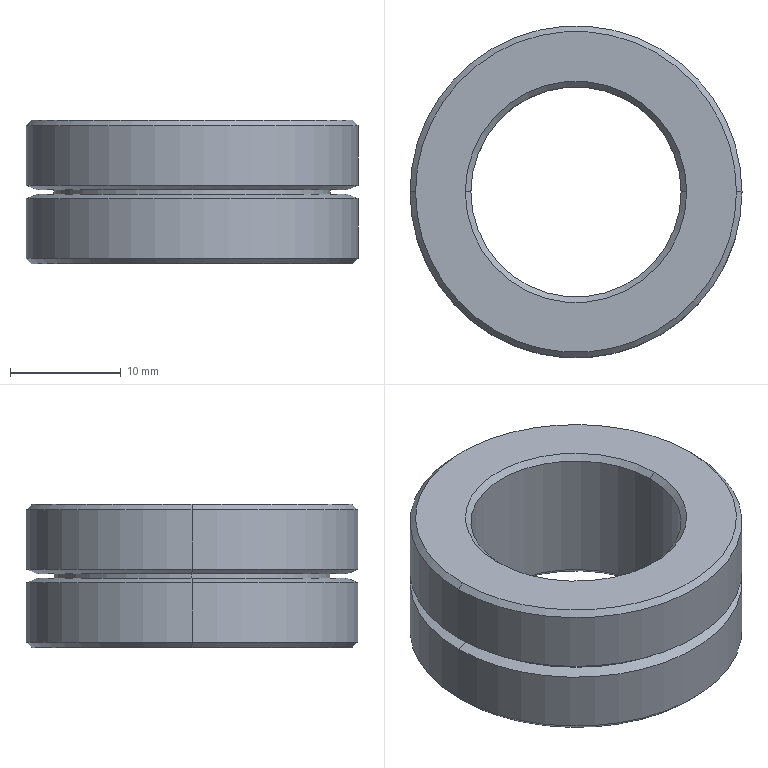Part | SolidWorks | features DelFace 2, MoveFace 2, Chamfer 1, Extrusion 1, ICE 1, MirrorPattern 1, RevCut 1 | 1 solid | 24 faces | box 30 x 30 x 13 mm | volume 5342 mm3 | cone 12 | cylinder 8 | plane 4 | commonest cylinder face diameters 30 x4 19 x2 25 x2
STEP:
#1=CARTESIAN_POINT('',(14.,0.,0.2));
#2=VERTEX_POINT('',#1);
#3=CARTESIAN_POINT('',(-14.,0.,0.2));
#4=VERTEX_POINT('',#3);
#5=CARTESIAN_POINT('',(0.,0.,0.2));
#6=DIRECTION('',(0.,0.,1.));
#7=DIRECTION('',(1.,0.,0.));
#8=AXIS2_PLACEMENT_3D('',#5,#6,#7);
#9=CIRCLE('',#8,14.);
#10=EDGE_CURVE('',#2,#4,#9,.T.);
#11=ORIENTED_EDGE('',*,*,#10,.T.);
#12=CARTESIAN_POINT('',(-15.,0.,0.6));
#13=VERTEX_POINT('',#12);
#14=CARTESIAN_POINT('',(-14.,0.,0.2));
#15=DIRECTION('',(-0.9285,0.,0.3714));
#16=VECTOR('',#15,1000.);
#17=LINE('',#14,#16);
#18=EDGE_CURVE('',#4,#13,#17,.T.);
#19=ORIENTED_EDGE('',*,*,#18,.T.);
#20=CARTESIAN_POINT('',(15.,0.,0.6));
#21=VERTEX_POINT('',#20);
#22=CARTESIAN_POINT('',(0.,0.,0.6));
#23=DIRECTION('',(0.,0.,1.));
#24=DIRECTION('',(1.,0.,0.));
#25=AXIS2_PLACEMENT_3D('',#22,#23,#24);
#26=CIRCLE('',#25,15.);
#27=EDGE_CURVE('',#21,#13,#26,.T.);
#28=ORIENTED_EDGE('',*,*,#27,.F.);
#29=CARTESIAN_POINT('',(14.,0.,0.2));
#30=DIRECTION('',(0.9285,0.,0.3714));
#31=VECTOR('',#30,1000.);
#32=LINE('',#29,#31);
#33=EDGE_CURVE('',#2,#21,#32,.T.);
#34=ORIENTED_EDGE('',*,*,#33,.F.);
#35=EDGE_LOOP('',(#11,#19,#28,#34));
#36=FACE_OUTER_BOUND('',#35,.T.);
#37=CARTESIAN_POINT('',(0.,0.,0.2));
#38=DIRECTION('',(0.,0.,1.));
#39=DIRECTION('',(1.,0.,0.));
#40=AXIS2_PLACEMENT_3D('',#37,#38,#39);
#41=CONICAL_SURFACE('',#40,14.,1.19);
#42=ADVANCED_FACE('',(#36),#41,.T.);
#43=CARTESIAN_POINT('',(12.5,0.,-0.2));
#44=VERTEX_POINT('',#43);
#45=CARTESIAN_POINT('',(-12.5,0.,-0.2));
#46=VERTEX_POINT('',#45);
#47=CARTESIAN_POINT('',(0.,0.,-0.2));
#48=DIRECTION('',(0.,0.,1.));
#49=DIRECTION('',(1.,0.,0.));
#50=AXIS2_PLACEMENT_3D('',#47,#48,#49);
#51=CIRCLE('',#50,12.5);
#52=EDGE_CURVE('',#44,#46,#51,.T.);
#53=ORIENTED_EDGE('',*,*,#52,.T.);
#54=CARTESIAN_POINT('',(-12.5,0.,0.2));
#55=VERTEX_POINT('',#54);
#56=CARTESIAN_POINT('',(-12.5,0.,6.));
#57=DIRECTION('',(0.,0.,1.));
#58=VECTOR('',#57,1000.);
#59=LINE('',#56,#58);
#60=EDGE_CURVE('',#46,#55,#59,.T.);
#61=ORIENTED_EDGE('',*,*,#60,.T.);
#62=CARTESIAN_POINT('',(12.5,0.,0.2));
#63=VERTEX_POINT('',#62);
#64=CARTESIAN_POINT('',(0.,0.,0.2));
#65=DIRECTION('',(0.,0.,1.));
#66=DIRECTION('',(1.,0.,0.));
#67=AXIS2_PLACEMENT_3D('',#64,#65,#66);
#68=CIRCLE('',#67,12.5);
#69=EDGE_CURVE('',#63,#55,#68,.T.);
#70=ORIENTED_EDGE('',*,*,#69,.F.);
#71=CARTESIAN_POINT('',(12.5,0.,6.));
#72=DIRECTION('',(0.,0.,1.));
#73=VECTOR('',#72,1000.);
#74=LINE('',#71,#73);
#75=EDGE_CURVE('',#44,#63,#74,.T.);
#76=ORIENTED_EDGE('',*,*,#75,.F.);
#77=EDGE_LOOP('',(#53,#61,#70,#76));
#78=FACE_OUTER_BOUND('',#77,.T.);
#79=CARTESIAN_POINT('',(0.,0.,6.));
#80=DIRECTION('',(0.,0.,1.));
#81=DIRECTION('',(1.,0.,0.));
#82=AXIS2_PLACEMENT_3D('',#79,#80,#81);
#83=CYLINDRICAL_SURFACE('',#82,12.5);
#84=ADVANCED_FACE('',(#78),#83,.T.);
#85=CARTESIAN_POINT('',(14.,0.,-0.2));
#86=VERTEX_POINT('',#85);
#87=CARTESIAN_POINT('',(-14.,0.,-0.2));
#88=VERTEX_POINT('',#87);
#89=CARTESIAN_POINT('',(0.,0.,-0.2));
#90=DIRECTION('',(0.,0.,1.));
#91=DIRECTION('',(1.,0.,0.));
#92=AXIS2_PLACEMENT_3D('',#89,#90,#91);
#93=CIRCLE('',#92,14.);
#94=EDGE_CURVE('',#86,#88,#93,.T.);
#95=ORIENTED_EDGE('',*,*,#94,.F.);
#96=CARTESIAN_POINT('',(15.,0.,-0.6));
#97=VERTEX_POINT('',#96);
#98=CARTESIAN_POINT('',(15.,0.,-0.6));
#99=DIRECTION('',(0.9285,0.,-0.3714));
#100=VECTOR('',#99,1000.);
#101=LINE('',#98,#100);
#102=EDGE_CURVE('',#86,#97,#101,.T.);
#103=ORIENTED_EDGE('',*,*,#102,.T.);
#104=CARTESIAN_POINT('',(-15.,0.,-0.6));
#105=VERTEX_POINT('',#104);
#106=CARTESIAN_POINT('',(0.,0.,-0.6));
#107=DIRECTION('',(0.,0.,1.));
#108=DIRECTION('',(1.,0.,0.));
#109=AXIS2_PLACEMENT_3D('',#106,#107,#108);
#110=CIRCLE('',#109,15.);
#111=EDGE_CURVE('',#97,#105,#110,.T.);
#112=ORIENTED_EDGE('',*,*,#111,.T.);
#113=CARTESIAN_POINT('',(-15.,0.,-0.6));
#114=DIRECTION('',(-0.9285,0.,-0.3714));
#115=VECTOR('',#114,1000.);
#116=LINE('',#113,#115);
#117=EDGE_CURVE('',#88,#105,#116,.T.);
#118=ORIENTED_EDGE('',*,*,#117,.F.);
#119=EDGE_LOOP('',(#95,#103,#112,#118));
#120=FACE_OUTER_BOUND('',#119,.T.);
#121=CARTESIAN_POINT('',(0.,0.,-0.6));
#122=DIRECTION('',(0.,0.,-1.));
#123=DIRECTION('',(-1.,0.,0.));
#124=AXIS2_PLACEMENT_3D('',#121,#122,#123);
#125=CONICAL_SURFACE('',#124,15.,1.19);
#126=ADVANCED_FACE('',(#120),#125,.T.);
#127=CARTESIAN_POINT('',(-9.5,0.,6.));
#128=VERTEX_POINT('',#127);
#129=CARTESIAN_POINT('',(9.5,0.,6.));
#130=VERTEX_POINT('',#129);
#131=CARTESIAN_POINT('',(0.,0.,6.));
#132=DIRECTION('',(0.,0.,1.));
#133=DIRECTION('',(1.,0.,0.));
#134=AXIS2_PLACEMENT_3D('',#131,#132,#133);
#135=CIRCLE('',#134,9.5);
#136=EDGE_CURVE('',#128,#130,#135,.T.);
#137=ORIENTED_EDGE('',*,*,#136,.F.);
#138=CARTESIAN_POINT('',(-10.,0.,6.5));
#139=VERTEX_POINT('',#138);
#140=CARTESIAN_POINT('',(-9.5,0.,6.));
#141=DIRECTION('',(-0.7071,0.,0.7071));
#142=VECTOR('',#141,1000.);
#143=LINE('',#140,#142);
#144=EDGE_CURVE('',#128,#139,#143,.T.);
#145=ORIENTED_EDGE('',*,*,#144,.T.);
#146=CARTESIAN_POINT('',(10.,0.,6.5));
#147=VERTEX_POINT('',#146);
#148=CARTESIAN_POINT('',(0.,0.,6.5));
#149=DIRECTION('',(0.,0.,-1.));
#150=DIRECTION('',(1.,0.,0.));
#151=AXIS2_PLACEMENT_3D('',#148,#149,#150);
#152=CIRCLE('',#151,10.);
#153=EDGE_CURVE('',#147,#139,#152,.T.);
#154=ORIENTED_EDGE('',*,*,#153,.F.);
#155=CARTESIAN_POINT('',(9.5,0.,6.));
#156=DIRECTION('',(0.7071,0.,0.7071));
#157=VECTOR('',#156,1000.);
#158=LINE('',#155,#157);
#159=EDGE_CURVE('',#130,#147,#158,.T.);
#160=ORIENTED_EDGE('',*,*,#159,.F.);
#161=EDGE_LOOP('',(#137,#145,#154,#160));
#162=FACE_OUTER_BOUND('',#161,.T.);
#163=CARTESIAN_POINT('',(0.,0.,6.));
#164=DIRECTION('',(0.,0.,1.));
#165=DIRECTION('',(1.,0.,0.));
#166=AXIS2_PLACEMENT_3D('',#163,#164,#165);
#167=CONICAL_SURFACE('',#166,9.5,0.7854);
#168=ADVANCED_FACE('',(#162),#167,.F.);
#169=CARTESIAN_POINT('',(9.5,0.,-6.));
#170=VERTEX_POINT('',#169);
#171=CARTESIAN_POINT('',(-9.5,0.,-6.));
#172=VERTEX_POINT('',#171);
#173=CARTESIAN_POINT('',(0.,0.,-6.));
#174=DIRECTION('',(0.,0.,-1.));
#175=DIRECTION('',(1.,0.,0.));
#176=AXIS2_PLACEMENT_3D('',#173,#174,#175);
#177=CIRCLE('',#176,9.5);
#178=EDGE_CURVE('',#170,#172,#177,.T.);
#179=ORIENTED_EDGE('',*,*,#178,.F.);
#180=CARTESIAN_POINT('',(10.,0.,-6.5));
#181=VERTEX_POINT('',#180);
#182=CARTESIAN_POINT('',(10.,0.,-6.5));
#183=DIRECTION('',(0.7071,0.,-0.7071));
#184=VECTOR('',#183,1000.);
#185=LINE('',#182,#184);
#186=EDGE_CURVE('',#170,#181,#185,.T.);
#187=ORIENTED_EDGE('',*,*,#186,.T.);
#188=CARTESIAN_POINT('',(-10.,0.,-6.5));
#189=VERTEX_POINT('',#188);
#190=CARTESIAN_POINT('',(0.,0.,-6.5));
#191=DIRECTION('',(0.,0.,1.));
#192=DIRECTION('',(1.,0.,0.));
#193=AXIS2_PLACEMENT_3D('',#190,#191,#192);
#194=CIRCLE('',#193,10.);
#195=EDGE_CURVE('',#189,#181,#194,.T.);
#196=ORIENTED_EDGE('',*,*,#195,.F.);
#197=CARTESIAN_POINT('',(-10.,0.,-6.5));
#198=DIRECTION('',(-0.7071,0.,-0.7071));
#199=VECTOR('',#198,1000.);
#200=LINE('',#197,#199);
#201=EDGE_CURVE('',#172,#189,#200,.T.);
#202=ORIENTED_EDGE('',*,*,#201,.F.);
#203=EDGE_LOOP('',(#179,#187,#196,#202));
#204=FACE_OUTER_BOUND('',#203,.T.);
#205=CARTESIAN_POINT('',(0.,0.,-6.5));
#206=DIRECTION('',(0.,0.,-1.));
#207=DIRECTION('',(-1.,0.,0.));
#208=AXIS2_PLACEMENT_3D('',#205,#206,#207);
#209=CONICAL_SURFACE('',#208,10.,0.7854);
#210=ADVANCED_FACE('',(#204),#209,.F.);
#211=CARTESIAN_POINT('',(14.5,0.,6.5));
#212=VERTEX_POINT('',#211);
#213=CARTESIAN_POINT('',(-14.5,0.,6.5));
#214=VERTEX_POINT('',#213);
#215=CARTESIAN_POINT('',(0.,0.,6.5));
#216=DIRECTION('',(0.,0.,1.));
#217=DIRECTION('',(1.,0.,0.));
#218=AXIS2_PLACEMENT_3D('',#215,#216,#217);
#219=CIRCLE('',#218,14.5);
#220=EDGE_CURVE('',#212,#214,#219,.T.);
#221=ORIENTED_EDGE('',*,*,#220,.F.);
#222=CARTESIAN_POINT('',(15.,0.,6.));
#223=VERTEX_POINT('',#222);
#224=CARTESIAN_POINT('',(14.5,0.,6.5));
#225=DIRECTION('',(0.7071,0.,-0.7071));
#226=VECTOR('',#225,1000.);
#227=LINE('',#224,#226);
#228=EDGE_CURVE('',#212,#223,#227,.T.);
#229=ORIENTED_EDGE('',*,*,#228,.T.);
#230=CARTESIAN_POINT('',(-15.,0.,6.));
#231=VERTEX_POINT('',#230);
#232=CARTESIAN_POINT('',(0.,0.,6.));
#233=DIRECTION('',(0.,0.,-1.));
#234=DIRECTION('',(1.,0.,0.));
#235=AXIS2_PLACEMENT_3D('',#232,#233,#234);
#236=CIRCLE('',#235,15.);
#237=EDGE_CURVE('',#231,#223,#236,.T.);
#238=ORIENTED_EDGE('',*,*,#237,.F.);
#239=CARTESIAN_POINT('',(-14.5,0.,6.5));
#240=DIRECTION('',(-0.7071,0.,-0.7071));
#241=VECTOR('',#240,1000.);
#242=LINE('',#239,#241);
#243=EDGE_CURVE('',#214,#231,#242,.T.);
#244=ORIENTED_EDGE('',*,*,#243,.F.);
#245=EDGE_LOOP('',(#221,#229,#238,#244));
#246=FACE_OUTER_BOUND('',#245,.T.);
#247=CARTESIAN_POINT('',(0.,0.,6.5));
#248=DIRECTION('',(0.,0.,-1.));
#249=DIRECTION('',(-1.,0.,0.));
#250=AXIS2_PLACEMENT_3D('',#247,#248,#249);
#251=CONICAL_SURFACE('',#250,14.5,0.7854);
#252=ADVANCED_FACE('',(#246),#251,.T.);
#253=CARTESIAN_POINT('',(-14.5,0.,-6.5));
#254=VERTEX_POINT('',#253);
#255=CARTESIAN_POINT('',(14.5,0.,-6.5));
#256=VERTEX_POINT('',#255);
#257=CARTESIAN_POINT('',(0.,0.,-6.5));
#258=DIRECTION('',(0.,0.,-1.));
#259=DIRECTION('',(1.,0.,0.));
#260=AXIS2_PLACEMENT_3D('',#257,#258,#259);
#261=CIRCLE('',#260,14.5);
#262=EDGE_CURVE('',#254,#256,#261,.T.);
#263=ORIENTED_EDGE('',*,*,#262,.F.);
#264=CARTESIAN_POINT('',(-15.,0.,-6.));
#265=VERTEX_POINT('',#264);
#266=CARTESIAN_POINT('',(-15.,0.,-6.));
#267=DIRECTION('',(-0.7071,0.,0.7071));
#268=VECTOR('',#267,1000.);
#269=LINE('',#266,#268);
#270=EDGE_CURVE('',#254,#265,#269,.T.);
#271=ORIENTED_EDGE('',*,*,#270,.T.);
#272=CARTESIAN_POINT('',(15.,0.,-6.));
#273=VERTEX_POINT('',#272);
#274=CARTESIAN_POINT('',(0.,0.,-6.));
#275=DIRECTION('',(0.,0.,1.));
#276=DIRECTION('',(1.,0.,0.));
#277=AXIS2_PLACEMENT_3D('',#274,#275,#276);
#278=CIRCLE('',#277,15.);
#279=EDGE_CURVE('',#273,#265,#278,.T.);
#280=ORIENTED_EDGE('',*,*,#279,.F.);
#281=CARTESIAN_POINT('',(15.,0.,-6.));
#282=DIRECTION('',(0.7071,0.,0.7071));
#283=VECTOR('',#282,1000.);
#284=LINE('',#281,#283);
#285=EDGE_CURVE('',#256,#273,#284,.T.);
#286=ORIENTED_EDGE('',*,*,#285,.F.);
#287=EDGE_LOOP('',(#263,#271,#280,#286));
#288=FACE_OUTER_BOUND('',#287,.T.);
#289=CARTESIAN_POINT('',(0.,0.,-6.));
#290=DIRECTION('',(0.,0.,1.));
#291=DIRECTION('',(1.,0.,0.));
#292=AXIS2_PLACEMENT_3D('',#289,#290,#291);
#293=CONICAL_SURFACE('',#292,15.,0.7854);
#294=ADVANCED_FACE('',(#288),#293,.T.);
#295=ORIENTED_EDGE('',*,*,#136,.T.);
#296=CARTESIAN_POINT('',(9.5,0.,8.));
#297=DIRECTION('',(0.,0.,-1.));
#298=VECTOR('',#297,1000.);
#299=LINE('',#296,#298);
#300=EDGE_CURVE('',#130,#170,#299,.T.);
#301=ORIENTED_EDGE('',*,*,#300,.T.);
#302=ORIENTED_EDGE('',*,*,#178,.T.);
#303=CARTESIAN_POINT('',(-9.5,0.,8.));
#304=DIRECTION('',(0.,0.,-1.));
#305=VECTOR('',#304,1000.);
#306=LINE('',#303,#305);
#307=EDGE_CURVE('',#128,#172,#306,.T.);
#308=ORIENTED_EDGE('',*,*,#307,.F.);
#309=EDGE_LOOP('',(#295,#301,#302,#308));
#310=FACE_OUTER_BOUND('',#309,.T.);
#311=CARTESIAN_POINT('',(0.,0.,8.));
#312=DIRECTION('',(0.,0.,-1.));
#313=DIRECTION('',(-1.,0.,0.));
#314=AXIS2_PLACEMENT_3D('',#311,#312,#313);
#315=CYLINDRICAL_SURFACE('',#314,9.5);
#316=ADVANCED_FACE('',(#310),#315,.F.);
#317=ORIENTED_EDGE('',*,*,#237,.T.);
#318=CARTESIAN_POINT('',(15.,0.,8.));
#319=DIRECTION('',(0.,0.,-1.));
#320=VECTOR('',#319,1000.);
#321=LINE('',#318,#320);
#322=EDGE_CURVE('',#223,#21,#321,.T.);
#323=ORIENTED_EDGE('',*,*,#322,.T.);
#324=ORIENTED_EDGE('',*,*,#27,.T.);
#325=CARTESIAN_POINT('',(-15.,0.,8.));
#326=DIRECTION('',(0.,0.,-1.));
#327=VECTOR('',#326,1000.);
#328=LINE('',#325,#327);
#329=EDGE_CURVE('',#231,#13,#328,.T.);
#330=ORIENTED_EDGE('',*,*,#329,.F.);
#331=EDGE_LOOP('',(#317,#323,#324,#330));
#332=FACE_OUTER_BOUND('',#331,.T.);
#333=CARTESIAN_POINT('',(0.,0.,8.));
#334=DIRECTION('',(0.,0.,-1.));
#335=DIRECTION('',(-1.,0.,0.));
#336=AXIS2_PLACEMENT_3D('',#333,#334,#335);
#337=CYLINDRICAL_SURFACE('',#336,15.);
#338=ADVANCED_FACE('',(#332),#337,.T.);
#339=ORIENTED_EDGE('',*,*,#111,.F.);
#340=CARTESIAN_POINT('',(15.,0.,8.));
#341=DIRECTION('',(0.,0.,-1.));
#342=VECTOR('',#341,1000.);
#343=LINE('',#340,#342);
#344=EDGE_CURVE('',#97,#273,#343,.T.);
#345=ORIENTED_EDGE('',*,*,#344,.T.);
#346=ORIENTED_EDGE('',*,*,#279,.T.);
#347=CARTESIAN_POINT('',(-15.,0.,8.));
#348=DIRECTION('',(0.,0.,-1.));
#349=VECTOR('',#348,1000.);
#350=LINE('',#347,#349);
#351=EDGE_CURVE('',#105,#265,#350,.T.);
#352=ORIENTED_EDGE('',*,*,#351,.F.);
#353=EDGE_LOOP('',(#339,#345,#346,#352));
#354=FACE_OUTER_BOUND('',#353,.T.);
#355=CARTESIAN_POINT('',(0.,0.,8.));
#356=DIRECTION('',(0.,0.,-1.));
#357=DIRECTION('',(-1.,0.,0.));
#358=AXIS2_PLACEMENT_3D('',#355,#356,#357);
#359=CYLINDRICAL_SURFACE('',#358,15.);
#360=ADVANCED_FACE('',(#354),#359,.T.);
#361=ORIENTED_EDGE('',*,*,#344,.F.);
#362=CARTESIAN_POINT('',(0.,0.,-0.6));
#363=DIRECTION('',(0.,0.,1.));
#364=DIRECTION('',(1.,0.,0.));
#365=AXIS2_PLACEMENT_3D('',#362,#363,#364);
#366=CIRCLE('',#365,15.);
#367=EDGE_CURVE('',#105,#97,#366,.T.);
#368=ORIENTED_EDGE('',*,*,#367,.F.);
#369=ORIENTED_EDGE('',*,*,#351,.T.);
#370=CARTESIAN_POINT('',(0.,0.,-6.));
#371=DIRECTION('',(0.,0.,1.));
#372=DIRECTION('',(1.,0.,0.));
#373=AXIS2_PLACEMENT_3D('',#370,#371,#372);
#374=CIRCLE('',#373,15.);
#375=EDGE_CURVE('',#265,#273,#374,.T.);
#376=ORIENTED_EDGE('',*,*,#375,.T.);
#377=EDGE_LOOP('',(#361,#368,#369,#376));
#378=FACE_OUTER_BOUND('',#377,.T.);
#379=CARTESIAN_POINT('',(0.,0.,8.));
#380=DIRECTION('',(0.,0.,-1.));
#381=DIRECTION('',(-1.,0.,0.));
#382=AXIS2_PLACEMENT_3D('',#379,#380,#381);
#383=CYLINDRICAL_SURFACE('',#382,15.);
#384=ADVANCED_FACE('',(#378),#383,.T.);
#385=CARTESIAN_POINT('',(0.,0.,6.5));
#386=DIRECTION('',(0.,0.,1.));
#387=DIRECTION('',(1.,0.,0.));
#388=AXIS2_PLACEMENT_3D('',#385,#386,#387);
#389=CIRCLE('',#388,14.5);
#390=EDGE_CURVE('',#214,#212,#389,.T.);
#391=ORIENTED_EDGE('',*,*,#390,.T.);
#392=ORIENTED_EDGE('',*,*,#220,.T.);
#393=EDGE_LOOP('',(#391,#392));
#394=FACE_OUTER_BOUND('',#393,.T.);
#395=ORIENTED_EDGE('',*,*,#153,.T.);
#396=CARTESIAN_POINT('',(0.,0.,6.5));
#397=DIRECTION('',(0.,0.,-1.));
#398=DIRECTION('',(1.,0.,0.));
#399=AXIS2_PLACEMENT_3D('',#396,#397,#398);
#400=CIRCLE('',#399,10.);
#401=EDGE_CURVE('',#139,#147,#400,.T.);
#402=ORIENTED_EDGE('',*,*,#401,.T.);
#403=EDGE_LOOP('',(#395,#402));
#404=FACE_BOUND('',#403,.T.);
#405=CARTESIAN_POINT('',(0.,0.,6.5));
#406=DIRECTION('',(0.,0.,1.));
#407=DIRECTION('',(1.,0.,0.));
#408=AXIS2_PLACEMENT_3D('',#405,#406,#407);
#409=PLANE('',#408);
#410=ADVANCED_FACE('',(#394,#404),#409,.T.);
#411=CARTESIAN_POINT('',(0.,0.,-6.5));
#412=DIRECTION('',(0.,0.,-1.));
#413=DIRECTION('',(1.,0.,0.));
#414=AXIS2_PLACEMENT_3D('',#411,#412,#413);
#415=CIRCLE('',#414,14.5);
#416=EDGE_CURVE('',#256,#254,#415,.T.);
#417=ORIENTED_EDGE('',*,*,#416,.T.);
#418=ORIENTED_EDGE('',*,*,#262,.T.);
#419=EDGE_LOOP('',(#417,#418));
#420=FACE_OUTER_BOUND('',#419,.T.);
#421=ORIENTED_EDGE('',*,*,#195,.T.);
#422=CARTESIAN_POINT('',(0.,0.,-6.5));
#423=DIRECTION('',(0.,0.,1.));
#424=DIRECTION('',(1.,0.,0.));
#425=AXIS2_PLACEMENT_3D('',#422,#423,#424);
#426=CIRCLE('',#425,10.);
#427=EDGE_CURVE('',#181,#189,#426,.T.);
#428=ORIENTED_EDGE('',*,*,#427,.T.);
#429=EDGE_LOOP('',(#421,#428));
#430=FACE_BOUND('',#429,.T.);
#431=CARTESIAN_POINT('',(0.,0.,-6.5));
#432=DIRECTION('',(0.,0.,1.));
#433=DIRECTION('',(1.,0.,0.));
#434=AXIS2_PLACEMENT_3D('',#431,#432,#433);
#435=PLANE('',#434);
#436=ADVANCED_FACE('',(#420,#430),#435,.F.);
#437=ORIENTED_EDGE('',*,*,#322,.F.);
#438=CARTESIAN_POINT('',(0.,0.,6.));
#439=DIRECTION('',(0.,0.,-1.));
#440=DIRECTION('',(1.,0.,0.));
#441=AXIS2_PLACEMENT_3D('',#438,#439,#440);
#442=CIRCLE('',#441,15.);
#443=EDGE_CURVE('',#223,#231,#442,.T.);
#444=ORIENTED_EDGE('',*,*,#443,.T.);
#445=ORIENTED_EDGE('',*,*,#329,.T.);
#446=CARTESIAN_POINT('',(0.,0.,0.6));
#447=DIRECTION('',(0.,0.,1.));
#448=DIRECTION('',(1.,0.,0.));
#449=AXIS2_PLACEMENT_3D('',#446,#447,#448);
#450=CIRCLE('',#449,15.);
#451=EDGE_CURVE('',#13,#21,#450,.T.);
#452=ORIENTED_EDGE('',*,*,#451,.T.);
#453=EDGE_LOOP('',(#437,#444,#445,#452));
#454=FACE_OUTER_BOUND('',#453,.T.);
#455=CARTESIAN_POINT('',(0.,0.,8.));
#456=DIRECTION('',(0.,0.,-1.));
#457=DIRECTION('',(-1.,0.,0.));
#458=AXIS2_PLACEMENT_3D('',#455,#456,#457);
#459=CYLINDRICAL_SURFACE('',#458,15.);
#460=ADVANCED_FACE('',(#454),#459,.T.);
#461=ORIENTED_EDGE('',*,*,#300,.F.);
#462=CARTESIAN_POINT('',(0.,0.,6.));
#463=DIRECTION('',(0.,0.,1.));
#464=DIRECTION('',(1.,0.,0.));
#465=AXIS2_PLACEMENT_3D('',#462,#463,#464);
#466=CIRCLE('',#465,9.5);
#467=EDGE_CURVE('',#130,#128,#466,.T.);
#468=ORIENTED_EDGE('',*,*,#467,.T.);
#469=ORIENTED_EDGE('',*,*,#307,.T.);
#470=CARTESIAN_POINT('',(0.,0.,-6.));
#471=DIRECTION('',(0.,0.,-1.));
#472=DIRECTION('',(1.,0.,0.));
#473=AXIS2_PLACEMENT_3D('',#470,#471,#472);
#474=CIRCLE('',#473,9.5);
#475=EDGE_CURVE('',#172,#170,#474,.T.);
#476=ORIENTED_EDGE('',*,*,#475,.T.);
#477=EDGE_LOOP('',(#461,#468,#469,#476));
#478=FACE_OUTER_BOUND('',#477,.T.);
#479=CARTESIAN_POINT('',(0.,0.,8.));
#480=DIRECTION('',(0.,0.,-1.));
#481=DIRECTION('',(-1.,0.,0.));
#482=AXIS2_PLACEMENT_3D('',#479,#480,#481);
#483=CYLINDRICAL_SURFACE('',#482,9.5);
#484=ADVANCED_FACE('',(#478),#483,.F.);
#485=ORIENTED_EDGE('',*,*,#270,.F.);
#486=ORIENTED_EDGE('',*,*,#416,.F.);
#487=ORIENTED_EDGE('',*,*,#285,.T.);
#488=ORIENTED_EDGE('',*,*,#375,.F.);
#489=EDGE_LOOP('',(#485,#486,#487,#488));
#490=FACE_OUTER_BOUND('',#489,.T.);
#491=CARTESIAN_POINT('',(0.,0.,-6.));
#492=DIRECTION('',(0.,0.,1.));
#493=DIRECTION('',(1.,0.,0.));
#494=AXIS2_PLACEMENT_3D('',#491,#492,#493);
#495=CONICAL_SURFACE('',#494,15.,0.7854);
#496=ADVANCED_FACE('',(#490),#495,.T.);
#497=ORIENTED_EDGE('',*,*,#228,.F.);
#498=ORIENTED_EDGE('',*,*,#390,.F.);
#499=ORIENTED_EDGE('',*,*,#243,.T.);
#500=ORIENTED_EDGE('',*,*,#443,.F.);
#501=EDGE_LOOP('',(#497,#498,#499,#500));
#502=FACE_OUTER_BOUND('',#501,.T.);
#503=CARTESIAN_POINT('',(0.,0.,6.5));
#504=DIRECTION('',(0.,0.,-1.));
#505=DIRECTION('',(-1.,0.,0.));
#506=AXIS2_PLACEMENT_3D('',#503,#504,#505);
#507=CONICAL_SURFACE('',#506,14.5,0.7854);
#508=ADVANCED_FACE('',(#502),#507,.T.);
#509=ORIENTED_EDGE('',*,*,#186,.F.);
#510=ORIENTED_EDGE('',*,*,#475,.F.);
#511=ORIENTED_EDGE('',*,*,#201,.T.);
#512=ORIENTED_EDGE('',*,*,#427,.F.);
#513=EDGE_LOOP('',(#509,#510,#511,#512));
#514=FACE_OUTER_BOUND('',#513,.T.);
#515=CARTESIAN_POINT('',(0.,0.,-6.5));
#516=DIRECTION('',(0.,0.,-1.));
#517=DIRECTION('',(-1.,0.,0.));
#518=AXIS2_PLACEMENT_3D('',#515,#516,#517);
#519=CONICAL_SURFACE('',#518,10.,0.7854);
#520=ADVANCED_FACE('',(#514),#519,.F.);
#521=ORIENTED_EDGE('',*,*,#144,.F.);
#522=ORIENTED_EDGE('',*,*,#467,.F.);
#523=ORIENTED_EDGE('',*,*,#159,.T.);
#524=ORIENTED_EDGE('',*,*,#401,.F.);
#525=EDGE_LOOP('',(#521,#522,#523,#524));
#526=FACE_OUTER_BOUND('',#525,.T.);
#527=CARTESIAN_POINT('',(0.,0.,6.));
#528=DIRECTION('',(0.,0.,1.));
#529=DIRECTION('',(1.,0.,0.));
#530=AXIS2_PLACEMENT_3D('',#527,#528,#529);
#531=CONICAL_SURFACE('',#530,9.5,0.7854);
#532=ADVANCED_FACE('',(#526),#531,.F.);
#533=ORIENTED_EDGE('',*,*,#102,.F.);
#534=CARTESIAN_POINT('',(0.,0.,-0.2));
#535=DIRECTION('',(0.,0.,1.));
#536=DIRECTION('',(1.,0.,0.));
#537=AXIS2_PLACEMENT_3D('',#534,#535,#536);
#538=CIRCLE('',#537,14.);
#539=EDGE_CURVE('',#88,#86,#538,.T.);
#540=ORIENTED_EDGE('',*,*,#539,.F.);
#541=ORIENTED_EDGE('',*,*,#117,.T.);
#542=ORIENTED_EDGE('',*,*,#367,.T.);
#543=EDGE_LOOP('',(#533,#540,#541,#542));
#544=FACE_OUTER_BOUND('',#543,.T.);
#545=CARTESIAN_POINT('',(0.,0.,-0.6));
#546=DIRECTION('',(0.,0.,-1.));
#547=DIRECTION('',(-1.,0.,0.));
#548=AXIS2_PLACEMENT_3D('',#545,#546,#547);
#549=CONICAL_SURFACE('',#548,15.,1.19);
#550=ADVANCED_FACE('',(#544),#549,.T.);
#551=ORIENTED_EDGE('',*,*,#52,.F.);
#552=CARTESIAN_POINT('',(0.,0.,-0.2));
#553=DIRECTION('',(0.,0.,1.));
#554=DIRECTION('',(1.,0.,0.));
#555=AXIS2_PLACEMENT_3D('',#552,#553,#554);
#556=CIRCLE('',#555,12.5);
#557=EDGE_CURVE('',#46,#44,#556,.T.);
#558=ORIENTED_EDGE('',*,*,#557,.F.);
#559=EDGE_LOOP('',(#551,#558));
#560=FACE_BOUND('',#559,.T.);
#561=ORIENTED_EDGE('',*,*,#539,.T.);
#562=ORIENTED_EDGE('',*,*,#94,.T.);
#563=EDGE_LOOP('',(#561,#562));
#564=FACE_OUTER_BOUND('',#563,.T.);
#565=CARTESIAN_POINT('',(14.,0.,-0.2));
#566=DIRECTION('',(0.,0.,-1.));
#567=DIRECTION('',(-1.,0.,0.));
#568=AXIS2_PLACEMENT_3D('',#565,#566,#567);
#569=PLANE('',#568);
#570=ADVANCED_FACE('',(#560,#564),#569,.F.);
#571=ORIENTED_EDGE('',*,*,#60,.F.);
#572=ORIENTED_EDGE('',*,*,#557,.T.);
#573=ORIENTED_EDGE('',*,*,#75,.T.);
#574=CARTESIAN_POINT('',(0.,0.,0.2));
#575=DIRECTION('',(0.,0.,1.));
#576=DIRECTION('',(1.,0.,0.));
#577=AXIS2_PLACEMENT_3D('',#574,#575,#576);
#578=CIRCLE('',#577,12.5);
#579=EDGE_CURVE('',#55,#63,#578,.T.);
#580=ORIENTED_EDGE('',*,*,#579,.F.);
#581=EDGE_LOOP('',(#571,#572,#573,#580));
#582=FACE_OUTER_BOUND('',#581,.T.);
#583=CARTESIAN_POINT('',(0.,0.,6.));
#584=DIRECTION('',(0.,0.,1.));
#585=DIRECTION('',(1.,0.,0.));
#586=AXIS2_PLACEMENT_3D('',#583,#584,#585);
#587=CYLINDRICAL_SURFACE('',#586,12.5);
#588=ADVANCED_FACE('',(#582),#587,.T.);
#589=ORIENTED_EDGE('',*,*,#10,.F.);
#590=CARTESIAN_POINT('',(0.,0.,0.2));
#591=DIRECTION('',(0.,0.,1.));
#592=DIRECTION('',(1.,0.,0.));
#593=AXIS2_PLACEMENT_3D('',#590,#591,#592);
#594=CIRCLE('',#593,14.);
#595=EDGE_CURVE('',#4,#2,#594,.T.);
#596=ORIENTED_EDGE('',*,*,#595,.F.);
#597=EDGE_LOOP('',(#589,#596));
#598=FACE_OUTER_BOUND('',#597,.T.);
#599=ORIENTED_EDGE('',*,*,#69,.T.);
#600=ORIENTED_EDGE('',*,*,#579,.T.);
#601=EDGE_LOOP('',(#599,#600));
#602=FACE_BOUND('',#601,.T.);
#603=CARTESIAN_POINT('',(12.5,0.,0.2));
#604=DIRECTION('',(0.,0.,1.));
#605=DIRECTION('',(1.,0.,0.));
#606=AXIS2_PLACEMENT_3D('',#603,#604,#605);
#607=PLANE('',#606);
#608=ADVANCED_FACE('',(#598,#602),#607,.F.);
#609=ORIENTED_EDGE('',*,*,#18,.F.);
#610=ORIENTED_EDGE('',*,*,#595,.T.);
#611=ORIENTED_EDGE('',*,*,#33,.T.);
#612=ORIENTED_EDGE('',*,*,#451,.F.);
#613=EDGE_LOOP('',(#609,#610,#611,#612));
#614=FACE_OUTER_BOUND('',#613,.T.);
#615=CARTESIAN_POINT('',(0.,0.,0.2));
#616=DIRECTION('',(0.,0.,1.));
#617=DIRECTION('',(1.,0.,0.));
#618=AXIS2_PLACEMENT_3D('',#615,#616,#617);
#619=CONICAL_SURFACE('',#618,14.,1.19);
#620=ADVANCED_FACE('',(#614),#619,.T.);
#621=CLOSED_SHELL('',(#42,#84,#126,#168,#210,#252,#294,#316,#338,#360,#384,#410,#436,#460,#484,#496,#508,#520,#532,#550,#570,#588,#608,#620));
#622=MANIFOLD_SOLID_BREP('',#621);
#623=CARTESIAN_POINT('',(0.,0.,0.));
#624=DIRECTION('',(0.,0.,1.));
#625=DIRECTION('',(1.,0.,0.));
#626=AXIS2_PLACEMENT_3D('',#623,#624,#625);
#627=(LENGTH_UNIT()NAMED_UNIT(*)SI_UNIT(.MILLI.,.METRE.));
#628=UNCERTAINTY_MEASURE_WITH_UNIT(LENGTH_MEASURE(0.00001),#627,'','');
#629=(NAMED_UNIT(*)PLANE_ANGLE_UNIT()SI_UNIT($,.RADIAN.));
#630=(NAMED_UNIT(*)SI_UNIT($,.STERADIAN.)SOLID_ANGLE_UNIT());
#631=(GEOMETRIC_REPRESENTATION_CONTEXT(3)GLOBAL_UNCERTAINTY_ASSIGNED_CONTEXT((#628))GLOBAL_UNIT_ASSIGNED_CONTEXT((#627,#629,#630))REPRESENTATION_CONTEXT('',''));
#632=ADVANCED_BREP_SHAPE_REPRESENTATION('',(#622,#626),#631);